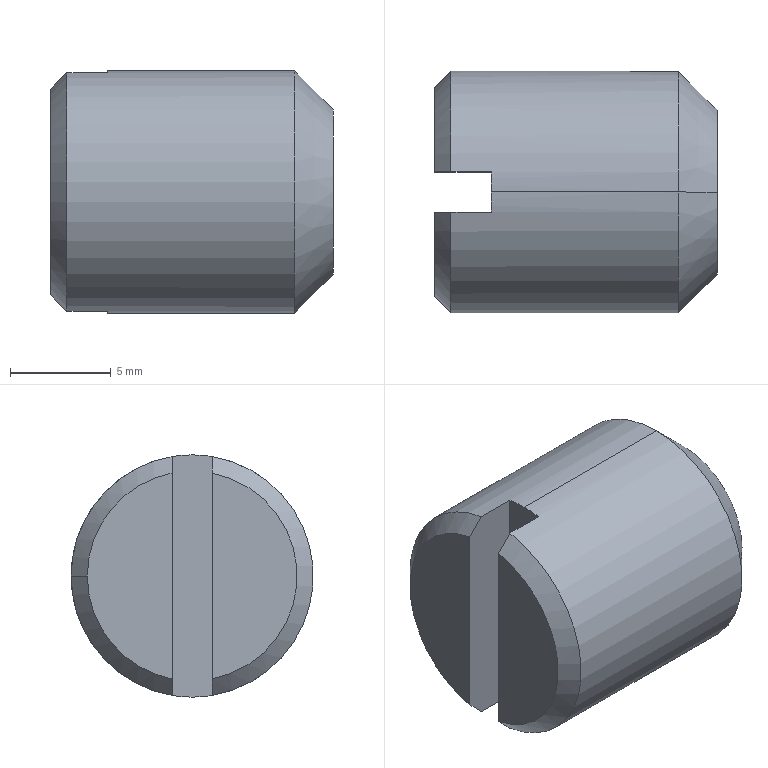Part | STEP file | 1 solid | 13 faces | box 14 x 12 x 12 mm | volume 1443 mm3 | plane 6 | cone 5 | cylinder 2 | commonest cylinder face diameters 12 x2
STEP:
#1=CARTESIAN_POINT('',(0.,0.,0.));
#2=DIRECTION('',(0.,0.,1.));
#3=DIRECTION('',(1.,0.,0.));
#4=AXIS2_PLACEMENT_3D('',#1,#2,#3);
#5=CARTESIAN_POINT('',(0.,1.,-5.099));
#6=VERTEX_POINT('',#5);
#7=CARTESIAN_POINT('',(0.,1.,5.099));
#8=VERTEX_POINT('',#7);
#9=CARTESIAN_POINT('',(0.,1.,-50.));
#10=DIRECTION('',(0.,0.,1.));
#11=VECTOR('',#10,1.);
#12=LINE('',#9,#11);
#13=CARTESIAN_POINT('',(0.,5.196,0.));
#14=DIRECTION('',(1.,0.,0.));
#15=DIRECTION('',(0.,1.,0.));
#16=AXIS2_PLACEMENT_3D('',#13,#14,#15);
#17=PLANE('',#16);
#18=CARTESIAN_POINT('',(-4.196,-50.));
#19=DIRECTION('',(0.,1.));
#20=VECTOR('',#19,1.);
#21=LINE('',#18,#20);
#22=(GEOMETRIC_REPRESENTATION_CONTEXT(2)PARAMETRIC_REPRESENTATION_CONTEXT()REPRESENTATION_CONTEXT('',''));
#23=DEFINITIONAL_REPRESENTATION('',(#21),#22);
#24=PCURVE('',#17,#23);
#25=CARTESIAN_POINT('',(0.,1.,-50.));
#26=DIRECTION('',(0.,1.,0.));
#27=DIRECTION('',(1.,0.,0.));
#28=AXIS2_PLACEMENT_3D('',#25,#26,#27);
#29=PLANE('',#28);
#30=CARTESIAN_POINT('',(0.,0.));
#31=DIRECTION('',(0.,-1.));
#32=VECTOR('',#31,1.);
#33=LINE('',#30,#32);
#34=(GEOMETRIC_REPRESENTATION_CONTEXT(2)PARAMETRIC_REPRESENTATION_CONTEXT()REPRESENTATION_CONTEXT('',''));
#35=DEFINITIONAL_REPRESENTATION('',(#33),#34);
#36=PCURVE('',#29,#35);
#37=SURFACE_CURVE('',#12,(#24,#36),.PCURVE_S1.);
#38=EDGE_CURVE('',#6,#8,#37,.T.);
#39=ORIENTED_EDGE('',*,*,#38,.T.);
#40=CARTESIAN_POINT('',(0.,5.196,0.));
#41=VERTEX_POINT('',#40);
#42=CARTESIAN_POINT('',(0.,0.,0.));
#43=DIRECTION('',(1.,0.,0.));
#44=DIRECTION('',(0.,1.,0.));
#45=AXIS2_PLACEMENT_3D('',#42,#43,#44);
#46=CIRCLE('',#45,5.196);
#47=CARTESIAN_POINT('',(-5.196,0.));
#48=DIRECTION('',(1.,0.));
#49=AXIS2_PLACEMENT_2D('',#47,#48);
#50=CIRCLE('',#49,5.196);
#51=(GEOMETRIC_REPRESENTATION_CONTEXT(2)PARAMETRIC_REPRESENTATION_CONTEXT()REPRESENTATION_CONTEXT('',''));
#52=DEFINITIONAL_REPRESENTATION('',(#50),#51);
#53=PCURVE('',#17,#52);
#54=CARTESIAN_POINT('',(0.804,0.,0.));
#55=DIRECTION('',(1.,0.,0.));
#56=DIRECTION('',(0.,1.,0.));
#57=AXIS2_PLACEMENT_3D('',#54,#55,#56);
#58=CONICAL_SURFACE('',#57,6.,0.7854);
#59=CARTESIAN_POINT('',(0.,-0.804));
#60=DIRECTION('',(1.,0.));
#61=VECTOR('',#60,1.);
#62=LINE('',#59,#61);
#63=(GEOMETRIC_REPRESENTATION_CONTEXT(2)PARAMETRIC_REPRESENTATION_CONTEXT()REPRESENTATION_CONTEXT('',''));
#64=DEFINITIONAL_REPRESENTATION('',(#62),#63);
#65=PCURVE('',#58,#64);
#66=SURFACE_CURVE('',#46,(#53,#65),.PCURVE_S1.);
#67=EDGE_CURVE('',#41,#8,#66,.T.);
#68=ORIENTED_EDGE('',*,*,#67,.F.);
#69=CARTESIAN_POINT('',(0.,0.,0.));
#70=DIRECTION('',(1.,0.,0.));
#71=DIRECTION('',(0.,1.,0.));
#72=AXIS2_PLACEMENT_3D('',#69,#70,#71);
#73=CIRCLE('',#72,5.196);
#74=CARTESIAN_POINT('',(-5.196,0.));
#75=DIRECTION('',(1.,0.));
#76=AXIS2_PLACEMENT_2D('',#74,#75);
#77=CIRCLE('',#76,5.196);
#78=(GEOMETRIC_REPRESENTATION_CONTEXT(2)PARAMETRIC_REPRESENTATION_CONTEXT()REPRESENTATION_CONTEXT('',''));
#79=DEFINITIONAL_REPRESENTATION('',(#77),#78);
#80=PCURVE('',#17,#79);
#81=CARTESIAN_POINT('',(0.804,0.,0.));
#82=DIRECTION('',(1.,0.,0.));
#83=DIRECTION('',(0.,1.,0.));
#84=AXIS2_PLACEMENT_3D('',#81,#82,#83);
#85=CONICAL_SURFACE('',#84,6.,0.7854);
#86=CARTESIAN_POINT('',(0.,-0.804));
#87=DIRECTION('',(1.,0.));
#88=VECTOR('',#87,1.);
#89=LINE('',#86,#88);
#90=(GEOMETRIC_REPRESENTATION_CONTEXT(2)PARAMETRIC_REPRESENTATION_CONTEXT()REPRESENTATION_CONTEXT('',''));
#91=DEFINITIONAL_REPRESENTATION('',(#89),#90);
#92=PCURVE('',#85,#91);
#93=SURFACE_CURVE('',#73,(#80,#92),.PCURVE_S1.);
#94=EDGE_CURVE('',#6,#41,#93,.T.);
#95=ORIENTED_EDGE('',*,*,#94,.F.);
#96=EDGE_LOOP('',(#39,#68,#95));
#97=FACE_BOUND('',#96,.T.);
#98=ADVANCED_FACE('',(#97),#17,.F.);
#99=CARTESIAN_POINT('',(14.,0.,4.07));
#100=VERTEX_POINT('',#99);
#101=CARTESIAN_POINT('',(14.,0.,-4.07));
#102=VERTEX_POINT('',#101);
#103=CARTESIAN_POINT('',(14.,0.,0.));
#104=DIRECTION('',(-1.,0.,0.));
#105=DIRECTION('',(0.,0.,1.));
#106=AXIS2_PLACEMENT_3D('',#103,#104,#105);
#107=CIRCLE('',#106,4.07);
#108=CARTESIAN_POINT('',(14.,0.,0.));
#109=DIRECTION('',(-1.,0.,0.));
#110=DIRECTION('',(0.,0.,1.));
#111=AXIS2_PLACEMENT_3D('',#108,#109,#110);
#112=PLANE('',#111);
#113=CARTESIAN_POINT('',(0.,0.));
#114=DIRECTION('',(1.,0.));
#115=AXIS2_PLACEMENT_2D('',#113,#114);
#116=CIRCLE('',#115,4.07);
#117=(GEOMETRIC_REPRESENTATION_CONTEXT(2)PARAMETRIC_REPRESENTATION_CONTEXT()REPRESENTATION_CONTEXT('',''));
#118=DEFINITIONAL_REPRESENTATION('',(#116),#117);
#119=PCURVE('',#112,#118);
#120=CARTESIAN_POINT('',(12.07,0.,0.));
#121=DIRECTION('',(-1.,0.,0.));
#122=DIRECTION('',(0.,0.,1.));
#123=AXIS2_PLACEMENT_3D('',#120,#121,#122);
#124=CONICAL_SURFACE('',#123,6.,0.7854);
#125=CARTESIAN_POINT('',(0.,-1.93));
#126=DIRECTION('',(1.,0.));
#127=VECTOR('',#126,1.);
#128=LINE('',#125,#127);
#129=(GEOMETRIC_REPRESENTATION_CONTEXT(2)PARAMETRIC_REPRESENTATION_CONTEXT()REPRESENTATION_CONTEXT('',''));
#130=DEFINITIONAL_REPRESENTATION('',(#128),#129);
#131=PCURVE('',#124,#130);
#132=SURFACE_CURVE('',#107,(#119,#131),.PCURVE_S1.);
#133=EDGE_CURVE('',#100,#102,#132,.T.);
#134=ORIENTED_EDGE('',*,*,#133,.F.);
#135=CARTESIAN_POINT('',(14.,0.,0.));
#136=DIRECTION('',(-1.,0.,0.));
#137=DIRECTION('',(0.,0.,1.));
#138=AXIS2_PLACEMENT_3D('',#135,#136,#137);
#139=CIRCLE('',#138,4.07);
#140=CARTESIAN_POINT('',(0.,0.));
#141=DIRECTION('',(1.,0.));
#142=AXIS2_PLACEMENT_2D('',#140,#141);
#143=CIRCLE('',#142,4.07);
#144=(GEOMETRIC_REPRESENTATION_CONTEXT(2)PARAMETRIC_REPRESENTATION_CONTEXT()REPRESENTATION_CONTEXT('',''));
#145=DEFINITIONAL_REPRESENTATION('',(#143),#144);
#146=PCURVE('',#112,#145);
#147=CARTESIAN_POINT('',(12.07,0.,0.));
#148=DIRECTION('',(-1.,0.,0.));
#149=DIRECTION('',(0.,0.,1.));
#150=AXIS2_PLACEMENT_3D('',#147,#148,#149);
#151=CONICAL_SURFACE('',#150,6.,0.7854);
#152=CARTESIAN_POINT('',(0.,-1.93));
#153=DIRECTION('',(1.,0.));
#154=VECTOR('',#153,1.);
#155=LINE('',#152,#154);
#156=(GEOMETRIC_REPRESENTATION_CONTEXT(2)PARAMETRIC_REPRESENTATION_CONTEXT()REPRESENTATION_CONTEXT('',''));
#157=DEFINITIONAL_REPRESENTATION('',(#155),#156);
#158=PCURVE('',#151,#157);
#159=SURFACE_CURVE('',#139,(#146,#158),.PCURVE_S1.);
#160=EDGE_CURVE('',#102,#100,#159,.T.);
#161=ORIENTED_EDGE('',*,*,#160,.F.);
#162=EDGE_LOOP('',(#134,#161));
#163=FACE_BOUND('',#162,.T.);
#164=ADVANCED_FACE('',(#163),#112,.F.);
#165=CARTESIAN_POINT('',(0.804,6.,0.));
#166=VERTEX_POINT('',#165);
#167=CARTESIAN_POINT('',(0.804,6.,0.));
#168=DIRECTION('',(0.7071,0.7071,0.));
#169=VECTOR('',#168,1.);
#170=LINE('',#167,#169);
#171=CARTESIAN_POINT('',(0.,0.));
#172=DIRECTION('',(0.,1.));
#173=VECTOR('',#172,1.);
#174=LINE('',#171,#173);
#175=(GEOMETRIC_REPRESENTATION_CONTEXT(2)PARAMETRIC_REPRESENTATION_CONTEXT()REPRESENTATION_CONTEXT('',''));
#176=DEFINITIONAL_REPRESENTATION('',(#174),#175);
#177=PCURVE('',#58,#176);
#178=CARTESIAN_POINT('',(6.283,0.));
#179=DIRECTION('',(0.,1.));
#180=VECTOR('',#179,1.);
#181=LINE('',#178,#180);
#182=(GEOMETRIC_REPRESENTATION_CONTEXT(2)PARAMETRIC_REPRESENTATION_CONTEXT()REPRESENTATION_CONTEXT('',''));
#183=DEFINITIONAL_REPRESENTATION('',(#181),#182);
#184=PCURVE('',#85,#183);
#185=SURFACE_CURVE('',#170,(#177,#184),.PCURVE_S1.);
#186=EDGE_CURVE('',#41,#166,#185,.T.);
#187=ORIENTED_EDGE('',*,*,#186,.F.);
#188=ORIENTED_EDGE('',*,*,#67,.T.);
#189=CARTESIAN_POINT('',(0.804,1.,5.916));
#190=VERTEX_POINT('',#189);
#191=CARTESIAN_POINT('',(0.,1.,5.099));
#192=CARTESIAN_POINT('',(0.2677,1.,5.372));
#193=CARTESIAN_POINT('',(0.5357,1.,5.644));
#194=CARTESIAN_POINT('',(0.804,1.,5.916));
#195=B_SPLINE_CURVE_WITH_KNOTS('',3,(#191,#192,#193,#194),.UNSPECIFIED.,.F.,.F.,(4,4),(0.,0.001146),.PIECEWISE_BEZIER_KNOTS.);
#196=CARTESIAN_POINT('',(1.377,-0.804));
#197=CARTESIAN_POINT('',(1.378,-0.7918));
#198=CARTESIAN_POINT('',(1.379,-0.7675));
#199=CARTESIAN_POINT('',(1.38,-0.731));
#200=CARTESIAN_POINT('',(1.381,-0.6945));
#201=CARTESIAN_POINT('',(1.382,-0.658));
#202=CARTESIAN_POINT('',(1.384,-0.6215));
#203=CARTESIAN_POINT('',(1.385,-0.5849));
#204=CARTESIAN_POINT('',(1.386,-0.5484));
#205=CARTESIAN_POINT('',(1.388,-0.5119));
#206=CARTESIAN_POINT('',(1.389,-0.4753));
#207=CARTESIAN_POINT('',(1.39,-0.4388));
#208=CARTESIAN_POINT('',(1.391,-0.4022));
#209=CARTESIAN_POINT('',(1.392,-0.3657));
#210=CARTESIAN_POINT('',(1.394,-0.3291));
#211=CARTESIAN_POINT('',(1.395,-0.2926));
#212=CARTESIAN_POINT('',(1.396,-0.256));
#213=CARTESIAN_POINT('',(1.397,-0.2195));
#214=CARTESIAN_POINT('',(1.398,-0.1829));
#215=CARTESIAN_POINT('',(1.399,-0.1463));
#216=CARTESIAN_POINT('',(1.4,-0.1097));
#217=CARTESIAN_POINT('',(1.401,-0.07317));
#218=CARTESIAN_POINT('',(1.402,-0.03659));
#219=CARTESIAN_POINT('',(1.403,-0.0122));
#220=CARTESIAN_POINT('',(1.403,0.));
#221=B_SPLINE_CURVE_WITH_KNOTS('',3,(#196,#197,#198,#199,#200,#201,#202,#203,#204,#205,#206,#207,#208,#209,#210,#211,#212,#213,#214,#215,#216,#217,#218,#219,#220),.UNSPECIFIED.,.F.,.F.,(4,1,1,1,1,1,1,1,1,1,1,1,1,1,1,1,1,1,1,1,1,1,4),(0.,0.00005211,0.0001042,0.0001563,0.0002084,0.0002605,0.0003127,0.0003648,0.0004169,0.000469,0.0005211,0.0005732,0.0006253,0.0006774,0.0007295,0.0007816,0.0008338,0.0008859,0.000938,0.0009901,0.001042,0.001094,0.001146),.QUASI_UNIFORM_KNOTS.);
#222=(GEOMETRIC_REPRESENTATION_CONTEXT(2)PARAMETRIC_REPRESENTATION_CONTEXT()REPRESENTATION_CONTEXT('',''));
#223=DEFINITIONAL_REPRESENTATION('',(#221),#222);
#224=PCURVE('',#58,#223);
#225=CARTESIAN_POINT('',(0.,-55.099));
#226=CARTESIAN_POINT('',(0.2677,-55.372));
#227=CARTESIAN_POINT('',(0.5357,-55.644));
#228=CARTESIAN_POINT('',(0.804,-55.916));
#229=B_SPLINE_CURVE_WITH_KNOTS('',3,(#225,#226,#227,#228),.UNSPECIFIED.,.F.,.F.,(4,4),(0.,0.001146),.PIECEWISE_BEZIER_KNOTS.);
#230=(GEOMETRIC_REPRESENTATION_CONTEXT(2)PARAMETRIC_REPRESENTATION_CONTEXT()REPRESENTATION_CONTEXT('',''));
#231=DEFINITIONAL_REPRESENTATION('',(#229),#230);
#232=PCURVE('',#29,#231);
#233=SURFACE_CURVE('',#195,(#224,#232),.PCURVE_S1.);
#234=EDGE_CURVE('',#8,#190,#233,.T.);
#235=ORIENTED_EDGE('',*,*,#234,.T.);
#236=CARTESIAN_POINT('',(0.804,0.,0.));
#237=DIRECTION('',(1.,0.,0.));
#238=DIRECTION('',(0.,0.,1.));
#239=AXIS2_PLACEMENT_3D('',#236,#237,#238);
#240=CIRCLE('',#239,6.);
#241=CARTESIAN_POINT('',(-4.712,0.));
#242=DIRECTION('',(1.,0.));
#243=VECTOR('',#242,1.);
#244=LINE('',#241,#243);
#245=(GEOMETRIC_REPRESENTATION_CONTEXT(2)PARAMETRIC_REPRESENTATION_CONTEXT()REPRESENTATION_CONTEXT('',''));
#246=DEFINITIONAL_REPRESENTATION('',(#244),#245);
#247=PCURVE('',#58,#246);
#248=CARTESIAN_POINT('',(-0.5499,0.,0.));
#249=DIRECTION('',(-1.,0.,0.));
#250=DIRECTION('',(0.,0.,1.));
#251=AXIS2_PLACEMENT_3D('',#248,#249,#250);
#252=CYLINDRICAL_SURFACE('',#251,6.);
#253=CARTESIAN_POINT('',(6.283,-1.354));
#254=DIRECTION('',(-1.,0.));
#255=VECTOR('',#254,1.);
#256=LINE('',#253,#255);
#257=(GEOMETRIC_REPRESENTATION_CONTEXT(2)PARAMETRIC_REPRESENTATION_CONTEXT()REPRESENTATION_CONTEXT('',''));
#258=DEFINITIONAL_REPRESENTATION('',(#256),#257);
#259=PCURVE('',#252,#258);
#260=SURFACE_CURVE('',#240,(#247,#259),.PCURVE_S1.);
#261=EDGE_CURVE('',#166,#190,#260,.T.);
#262=ORIENTED_EDGE('',*,*,#261,.F.);
#263=EDGE_LOOP('',(#187,#188,#235,#262));
#264=FACE_BOUND('',#263,.T.);
#265=ADVANCED_FACE('',(#264),#58,.T.);
#266=CARTESIAN_POINT('',(2.8,1.,5.916));
#267=VERTEX_POINT('',#266);
#268=CARTESIAN_POINT('',(-0.5499,1.,5.916));
#269=DIRECTION('',(1.,0.,0.));
#270=VECTOR('',#269,1.);
#271=LINE('',#268,#270);
#272=CARTESIAN_POINT('',(-0.5499,-55.916));
#273=DIRECTION('',(1.,0.));
#274=VECTOR('',#273,1.);
#275=LINE('',#272,#274);
#276=(GEOMETRIC_REPRESENTATION_CONTEXT(2)PARAMETRIC_REPRESENTATION_CONTEXT()REPRESENTATION_CONTEXT('',''));
#277=DEFINITIONAL_REPRESENTATION('',(#275),#276);
#278=PCURVE('',#29,#277);
#279=CARTESIAN_POINT('',(0.1674,0.));
#280=DIRECTION('',(0.,-1.));
#281=VECTOR('',#280,1.);
#282=LINE('',#279,#281);
#283=(GEOMETRIC_REPRESENTATION_CONTEXT(2)PARAMETRIC_REPRESENTATION_CONTEXT()REPRESENTATION_CONTEXT('',''));
#284=DEFINITIONAL_REPRESENTATION('',(#282),#283);
#285=PCURVE('',#252,#284);
#286=SURFACE_CURVE('',#271,(#278,#285),.PCURVE_S1.);
#287=EDGE_CURVE('',#190,#267,#286,.T.);
#288=ORIENTED_EDGE('',*,*,#287,.F.);
#289=ORIENTED_EDGE('',*,*,#234,.F.);
#290=ORIENTED_EDGE('',*,*,#38,.F.);
#291=CARTESIAN_POINT('',(0.804,1.,-5.916));
#292=VERTEX_POINT('',#291);
#293=CARTESIAN_POINT('',(0.804,1.,-5.916));
#294=CARTESIAN_POINT('',(0.5357,1.,-5.644));
#295=CARTESIAN_POINT('',(0.2677,1.,-5.372));
#296=CARTESIAN_POINT('',(0.,1.,-5.099));
#297=B_SPLINE_CURVE_WITH_KNOTS('',3,(#293,#294,#295,#296),.UNSPECIFIED.,.F.,.F.,(4,4),(0.,0.001146),.PIECEWISE_BEZIER_KNOTS.);
#298=CARTESIAN_POINT('',(0.804,-44.084));
#299=CARTESIAN_POINT('',(0.5357,-44.356));
#300=CARTESIAN_POINT('',(0.2677,-44.628));
#301=CARTESIAN_POINT('',(0.,-44.901));
#302=B_SPLINE_CURVE_WITH_KNOTS('',3,(#298,#299,#300,#301),.UNSPECIFIED.,.F.,.F.,(4,4),(0.,0.001146),.PIECEWISE_BEZIER_KNOTS.);
#303=(GEOMETRIC_REPRESENTATION_CONTEXT(2)PARAMETRIC_REPRESENTATION_CONTEXT()REPRESENTATION_CONTEXT('',''));
#304=DEFINITIONAL_REPRESENTATION('',(#302),#303);
#305=PCURVE('',#29,#304);
#306=CARTESIAN_POINT('',(4.88,0.));
#307=CARTESIAN_POINT('',(4.88,-0.0122));
#308=CARTESIAN_POINT('',(4.881,-0.03659));
#309=CARTESIAN_POINT('',(4.882,-0.07317));
#310=CARTESIAN_POINT('',(4.883,-0.1097));
#311=CARTESIAN_POINT('',(4.884,-0.1463));
#312=CARTESIAN_POINT('',(4.885,-0.1829));
#313=CARTESIAN_POINT('',(4.886,-0.2195));
#314=CARTESIAN_POINT('',(4.887,-0.256));
#315=CARTESIAN_POINT('',(4.889,-0.2926));
#316=CARTESIAN_POINT('',(4.89,-0.3291));
#317=CARTESIAN_POINT('',(4.891,-0.3657));
#318=CARTESIAN_POINT('',(4.892,-0.4022));
#319=CARTESIAN_POINT('',(4.893,-0.4388));
#320=CARTESIAN_POINT('',(4.894,-0.4753));
#321=CARTESIAN_POINT('',(4.896,-0.5119));
#322=CARTESIAN_POINT('',(4.897,-0.5484));
#323=CARTESIAN_POINT('',(4.898,-0.5849));
#324=CARTESIAN_POINT('',(4.899,-0.6215));
#325=CARTESIAN_POINT('',(4.901,-0.658));
#326=CARTESIAN_POINT('',(4.902,-0.6945));
#327=CARTESIAN_POINT('',(4.903,-0.731));
#328=CARTESIAN_POINT('',(4.905,-0.7675));
#329=CARTESIAN_POINT('',(4.906,-0.7918));
#330=CARTESIAN_POINT('',(4.906,-0.804));
#331=B_SPLINE_CURVE_WITH_KNOTS('',3,(#306,#307,#308,#309,#310,#311,#312,#313,#314,#315,#316,#317,#318,#319,#320,#321,#322,#323,#324,#325,#326,#327,#328,#329,#330),.UNSPECIFIED.,.F.,.F.,(4,1,1,1,1,1,1,1,1,1,1,1,1,1,1,1,1,1,1,1,1,1,4),(0.,0.00005211,0.0001042,0.0001563,0.0002084,0.0002605,0.0003127,0.0003648,0.0004169,0.000469,0.0005211,0.0005732,0.0006253,0.0006774,0.0007295,0.0007816,0.0008338,0.0008859,0.000938,0.0009901,0.001042,0.001094,0.001146),.QUASI_UNIFORM_KNOTS.);
#332=(GEOMETRIC_REPRESENTATION_CONTEXT(2)PARAMETRIC_REPRESENTATION_CONTEXT()REPRESENTATION_CONTEXT('',''));
#333=DEFINITIONAL_REPRESENTATION('',(#331),#332);
#334=PCURVE('',#85,#333);
#335=SURFACE_CURVE('',#297,(#305,#334),.PCURVE_S1.);
#336=EDGE_CURVE('',#292,#6,#335,.T.);
#337=ORIENTED_EDGE('',*,*,#336,.F.);
#338=CARTESIAN_POINT('',(2.8,1.,-5.916));
#339=VERTEX_POINT('',#338);
#340=CARTESIAN_POINT('',(-0.5499,1.,-5.916));
#341=DIRECTION('',(-1.,0.,0.));
#342=VECTOR('',#341,1.);
#343=LINE('',#340,#342);
#344=CARTESIAN_POINT('',(-0.5499,-44.084));
#345=DIRECTION('',(-1.,0.));
#346=VECTOR('',#345,1.);
#347=LINE('',#344,#346);
#348=(GEOMETRIC_REPRESENTATION_CONTEXT(2)PARAMETRIC_REPRESENTATION_CONTEXT()REPRESENTATION_CONTEXT('',''));
#349=DEFINITIONAL_REPRESENTATION('',(#347),#348);
#350=PCURVE('',#29,#349);
#351=CARTESIAN_POINT('',(2.974,0.));
#352=DIRECTION('',(0.,1.));
#353=VECTOR('',#352,1.);
#354=LINE('',#351,#353);
#355=(GEOMETRIC_REPRESENTATION_CONTEXT(2)PARAMETRIC_REPRESENTATION_CONTEXT()REPRESENTATION_CONTEXT('',''));
#356=DEFINITIONAL_REPRESENTATION('',(#354),#355);
#357=PCURVE('',#252,#356);
#358=SURFACE_CURVE('',#343,(#350,#357),.PCURVE_S1.);
#359=EDGE_CURVE('',#339,#292,#358,.T.);
#360=ORIENTED_EDGE('',*,*,#359,.F.);
#361=CARTESIAN_POINT('',(2.8,1.,-50.));
#362=DIRECTION('',(0.,0.,1.));
#363=VECTOR('',#362,1.);
#364=LINE('',#361,#363);
#365=CARTESIAN_POINT('',(2.8,0.));
#366=DIRECTION('',(0.,-1.));
#367=VECTOR('',#366,1.);
#368=LINE('',#365,#367);
#369=(GEOMETRIC_REPRESENTATION_CONTEXT(2)PARAMETRIC_REPRESENTATION_CONTEXT()REPRESENTATION_CONTEXT('',''));
#370=DEFINITIONAL_REPRESENTATION('',(#368),#369);
#371=PCURVE('',#29,#370);
#372=CARTESIAN_POINT('',(2.8,-1.,-50.));
#373=DIRECTION('',(1.,0.,0.));
#374=DIRECTION('',(0.,1.,0.));
#375=AXIS2_PLACEMENT_3D('',#372,#373,#374);
#376=PLANE('',#375);
#377=CARTESIAN_POINT('',(2.,0.));
#378=DIRECTION('',(0.,1.));
#379=VECTOR('',#378,1.);
#380=LINE('',#377,#379);
#381=(GEOMETRIC_REPRESENTATION_CONTEXT(2)PARAMETRIC_REPRESENTATION_CONTEXT()REPRESENTATION_CONTEXT('',''));
#382=DEFINITIONAL_REPRESENTATION('',(#380),#381);
#383=PCURVE('',#376,#382);
#384=SURFACE_CURVE('',#364,(#371,#383),.PCURVE_S1.);
#385=EDGE_CURVE('',#339,#267,#384,.T.);
#386=ORIENTED_EDGE('',*,*,#385,.T.);
#387=EDGE_LOOP('',(#288,#289,#290,#337,#360,#386));
#388=FACE_BOUND('',#387,.T.);
#389=ADVANCED_FACE('',(#388),#29,.F.);
#390=CARTESIAN_POINT('',(0.,-1.,5.099));
#391=VERTEX_POINT('',#390);
#392=CARTESIAN_POINT('',(0.,-1.,-5.099));
#393=VERTEX_POINT('',#392);
#394=CARTESIAN_POINT('',(0.,-1.,-50.));
#395=DIRECTION('',(0.,0.,-1.));
#396=VECTOR('',#395,1.);
#397=LINE('',#394,#396);
#398=CARTESIAN_POINT('',(0.,5.196,0.));
#399=DIRECTION('',(1.,0.,0.));
#400=DIRECTION('',(0.,1.,0.));
#401=AXIS2_PLACEMENT_3D('',#398,#399,#400);
#402=PLANE('',#401);
#403=CARTESIAN_POINT('',(-6.196,-50.));
#404=DIRECTION('',(0.,-1.));
#405=VECTOR('',#404,1.);
#406=LINE('',#403,#405);
#407=(GEOMETRIC_REPRESENTATION_CONTEXT(2)PARAMETRIC_REPRESENTATION_CONTEXT()REPRESENTATION_CONTEXT('',''));
#408=DEFINITIONAL_REPRESENTATION('',(#406),#407);
#409=PCURVE('',#402,#408);
#410=CARTESIAN_POINT('',(0.,-1.,-50.));
#411=DIRECTION('',(0.,-1.,0.));
#412=DIRECTION('',(0.,0.,-1.));
#413=AXIS2_PLACEMENT_3D('',#410,#411,#412);
#414=PLANE('',#413);
#415=CARTESIAN_POINT('',(0.,0.));
#416=DIRECTION('',(1.,0.));
#417=VECTOR('',#416,1.);
#418=LINE('',#415,#417);
#419=(GEOMETRIC_REPRESENTATION_CONTEXT(2)PARAMETRIC_REPRESENTATION_CONTEXT()REPRESENTATION_CONTEXT('',''));
#420=DEFINITIONAL_REPRESENTATION('',(#418),#419);
#421=PCURVE('',#414,#420);
#422=SURFACE_CURVE('',#397,(#409,#421),.PCURVE_S1.);
#423=EDGE_CURVE('',#391,#393,#422,.T.);
#424=ORIENTED_EDGE('',*,*,#423,.T.);
#425=CARTESIAN_POINT('',(0.,0.,0.));
#426=DIRECTION('',(1.,0.,0.));
#427=DIRECTION('',(0.,1.,0.));
#428=AXIS2_PLACEMENT_3D('',#425,#426,#427);
#429=CIRCLE('',#428,5.196);
#430=CARTESIAN_POINT('',(-5.196,0.));
#431=DIRECTION('',(1.,0.));
#432=AXIS2_PLACEMENT_2D('',#430,#431);
#433=CIRCLE('',#432,5.196);
#434=(GEOMETRIC_REPRESENTATION_CONTEXT(2)PARAMETRIC_REPRESENTATION_CONTEXT()REPRESENTATION_CONTEXT('',''));
#435=DEFINITIONAL_REPRESENTATION('',(#433),#434);
#436=PCURVE('',#402,#435);
#437=CARTESIAN_POINT('',(0.804,0.,0.));
#438=DIRECTION('',(1.,0.,0.));
#439=DIRECTION('',(0.,1.,0.));
#440=AXIS2_PLACEMENT_3D('',#437,#438,#439);
#441=CONICAL_SURFACE('',#440,6.,0.7854);
#442=CARTESIAN_POINT('',(0.,-0.804));
#443=DIRECTION('',(1.,0.));
#444=VECTOR('',#443,1.);
#445=LINE('',#442,#444);
#446=(GEOMETRIC_REPRESENTATION_CONTEXT(2)PARAMETRIC_REPRESENTATION_CONTEXT()REPRESENTATION_CONTEXT('',''));
#447=DEFINITIONAL_REPRESENTATION('',(#445),#446);
#448=PCURVE('',#441,#447);
#449=SURFACE_CURVE('',#429,(#436,#448),.PCURVE_S1.);
#450=EDGE_CURVE('',#391,#393,#449,.T.);
#451=ORIENTED_EDGE('',*,*,#450,.F.);
#452=EDGE_LOOP('',(#424,#451));
#453=FACE_BOUND('',#452,.T.);
#454=ADVANCED_FACE('',(#453),#402,.F.);
#455=CARTESIAN_POINT('',(2.8,-1.,-5.916));
#456=VERTEX_POINT('',#455);
#457=CARTESIAN_POINT('',(2.8,0.,-6.));
#458=VERTEX_POINT('',#457);
#459=CARTESIAN_POINT('',(2.8,0.,0.));
#460=DIRECTION('',(1.,0.,0.));
#461=DIRECTION('',(0.,0.,1.));
#462=AXIS2_PLACEMENT_3D('',#459,#460,#461);
#463=CIRCLE('',#462,6.);
#464=CARTESIAN_POINT('',(1.,50.));
#465=DIRECTION('',(0.,1.));
#466=AXIS2_PLACEMENT_2D('',#464,#465);
#467=CIRCLE('',#466,6.);
#468=(GEOMETRIC_REPRESENTATION_CONTEXT(2)PARAMETRIC_REPRESENTATION_CONTEXT()REPRESENTATION_CONTEXT('',''));
#469=DEFINITIONAL_REPRESENTATION('',(#467),#468);
#470=PCURVE('',#376,#469);
#471=CARTESIAN_POINT('',(-0.5499,0.,0.));
#472=DIRECTION('',(-1.,0.,0.));
#473=DIRECTION('',(0.,0.,1.));
#474=AXIS2_PLACEMENT_3D('',#471,#472,#473);
#475=CYLINDRICAL_SURFACE('',#474,6.);
#476=CARTESIAN_POINT('',(6.283,-3.35));
#477=DIRECTION('',(-1.,0.));
#478=VECTOR('',#477,1.);
#479=LINE('',#476,#478);
#480=(GEOMETRIC_REPRESENTATION_CONTEXT(2)PARAMETRIC_REPRESENTATION_CONTEXT()REPRESENTATION_CONTEXT('',''));
#481=DEFINITIONAL_REPRESENTATION('',(#479),#480);
#482=PCURVE('',#475,#481);
#483=SURFACE_CURVE('',#463,(#470,#482),.PCURVE_S1.);
#484=EDGE_CURVE('',#456,#458,#483,.T.);
#485=ORIENTED_EDGE('',*,*,#484,.F.);
#486=CARTESIAN_POINT('',(2.8,-1.,5.916));
#487=VERTEX_POINT('',#486);
#488=CARTESIAN_POINT('',(2.8,-1.,-50.));
#489=DIRECTION('',(0.,0.,1.));
#490=VECTOR('',#489,1.);
#491=LINE('',#488,#490);
#492=CARTESIAN_POINT('',(0.,0.));
#493=DIRECTION('',(0.,1.));
#494=VECTOR('',#493,1.);
#495=LINE('',#492,#494);
#496=(GEOMETRIC_REPRESENTATION_CONTEXT(2)PARAMETRIC_REPRESENTATION_CONTEXT()REPRESENTATION_CONTEXT('',''));
#497=DEFINITIONAL_REPRESENTATION('',(#495),#496);
#498=PCURVE('',#376,#497);
#499=CARTESIAN_POINT('',(0.,2.8));
#500=DIRECTION('',(-1.,0.));
#501=VECTOR('',#500,1.);
#502=LINE('',#499,#501);
#503=(GEOMETRIC_REPRESENTATION_CONTEXT(2)PARAMETRIC_REPRESENTATION_CONTEXT()REPRESENTATION_CONTEXT('',''));
#504=DEFINITIONAL_REPRESENTATION('',(#502),#503);
#505=PCURVE('',#414,#504);
#506=SURFACE_CURVE('',#491,(#498,#505),.PCURVE_S1.);
#507=EDGE_CURVE('',#456,#487,#506,.T.);
#508=ORIENTED_EDGE('',*,*,#507,.T.);
#509=CARTESIAN_POINT('',(2.8,0.,6.));
#510=VERTEX_POINT('',#509);
#511=CARTESIAN_POINT('',(2.8,0.,0.));
#512=DIRECTION('',(1.,0.,0.));
#513=DIRECTION('',(0.,0.,1.));
#514=AXIS2_PLACEMENT_3D('',#511,#512,#513);
#515=CIRCLE('',#514,6.);
#516=CARTESIAN_POINT('',(1.,50.));
#517=DIRECTION('',(0.,1.));
#518=AXIS2_PLACEMENT_2D('',#516,#517);
#519=CIRCLE('',#518,6.);
#520=(GEOMETRIC_REPRESENTATION_CONTEXT(2)PARAMETRIC_REPRESENTATION_CONTEXT()REPRESENTATION_CONTEXT('',''));
#521=DEFINITIONAL_REPRESENTATION('',(#519),#520);
#522=PCURVE('',#376,#521);
#523=CARTESIAN_POINT('',(6.283,-3.35));
#524=DIRECTION('',(-1.,0.));
#525=VECTOR('',#524,1.);
#526=LINE('',#523,#525);
#527=(GEOMETRIC_REPRESENTATION_CONTEXT(2)PARAMETRIC_REPRESENTATION_CONTEXT()REPRESENTATION_CONTEXT('',''));
#528=DEFINITIONAL_REPRESENTATION('',(#526),#527);
#529=PCURVE('',#475,#528);
#530=SURFACE_CURVE('',#515,(#522,#529),.PCURVE_S1.);
#531=EDGE_CURVE('',#510,#487,#530,.T.);
#532=ORIENTED_EDGE('',*,*,#531,.F.);
#533=CARTESIAN_POINT('',(2.8,0.,0.));
#534=DIRECTION('',(1.,0.,0.));
#535=DIRECTION('',(0.,0.,1.));
#536=AXIS2_PLACEMENT_3D('',#533,#534,#535);
#537=CIRCLE('',#536,6.);
#538=CARTESIAN_POINT('',(1.,50.));
#539=DIRECTION('',(0.,1.));
#540=AXIS2_PLACEMENT_2D('',#538,#539);
#541=CIRCLE('',#540,6.);
#542=(GEOMETRIC_REPRESENTATION_CONTEXT(2)PARAMETRIC_REPRESENTATION_CONTEXT()REPRESENTATION_CONTEXT('',''));
#543=DEFINITIONAL_REPRESENTATION('',(#541),#542);
#544=PCURVE('',#376,#543);
#545=CARTESIAN_POINT('',(6.283,-3.35));
#546=DIRECTION('',(-1.,0.));
#547=VECTOR('',#546,1.);
#548=LINE('',#545,#547);
#549=(GEOMETRIC_REPRESENTATION_CONTEXT(2)PARAMETRIC_REPRESENTATION_CONTEXT()REPRESENTATION_CONTEXT('',''));
#550=DEFINITIONAL_REPRESENTATION('',(#548),#549);
#551=PCURVE('',#252,#550);
#552=SURFACE_CURVE('',#537,(#544,#551),.PCURVE_S1.);
#553=EDGE_CURVE('',#267,#510,#552,.T.);
#554=ORIENTED_EDGE('',*,*,#553,.F.);
#555=ORIENTED_EDGE('',*,*,#385,.F.);
#556=CARTESIAN_POINT('',(2.8,0.,0.));
#557=DIRECTION('',(1.,0.,0.));
#558=DIRECTION('',(0.,0.,1.));
#559=AXIS2_PLACEMENT_3D('',#556,#557,#558);
#560=CIRCLE('',#559,6.);
#561=CARTESIAN_POINT('',(1.,50.));
#562=DIRECTION('',(0.,1.));
#563=AXIS2_PLACEMENT_2D('',#561,#562);
#564=CIRCLE('',#563,6.);
#565=(GEOMETRIC_REPRESENTATION_CONTEXT(2)PARAMETRIC_REPRESENTATION_CONTEXT()REPRESENTATION_CONTEXT('',''));
#566=DEFINITIONAL_REPRESENTATION('',(#564),#565);
#567=PCURVE('',#376,#566);
#568=CARTESIAN_POINT('',(6.283,-3.35));
#569=DIRECTION('',(-1.,0.));
#570=VECTOR('',#569,1.);
#571=LINE('',#568,#570);
#572=(GEOMETRIC_REPRESENTATION_CONTEXT(2)PARAMETRIC_REPRESENTATION_CONTEXT()REPRESENTATION_CONTEXT('',''));
#573=DEFINITIONAL_REPRESENTATION('',(#571),#572);
#574=PCURVE('',#252,#573);
#575=SURFACE_CURVE('',#560,(#567,#574),.PCURVE_S1.);
#576=EDGE_CURVE('',#458,#339,#575,.T.);
#577=ORIENTED_EDGE('',*,*,#576,.F.);
#578=EDGE_LOOP('',(#485,#508,#532,#554,#555,#577));
#579=FACE_BOUND('',#578,.T.);
#580=ADVANCED_FACE('',(#579),#376,.F.);
#581=CARTESIAN_POINT('',(12.07,0.,-6.));
#582=VERTEX_POINT('',#581);
#583=CARTESIAN_POINT('',(12.07,0.,-6.));
#584=DIRECTION('',(-0.7071,0.,-0.7071));
#585=VECTOR('',#584,1.);
#586=LINE('',#583,#585);
#587=CARTESIAN_POINT('',(3.142,0.));
#588=DIRECTION('',(0.,1.));
#589=VECTOR('',#588,1.);
#590=LINE('',#587,#589);
#591=(GEOMETRIC_REPRESENTATION_CONTEXT(2)PARAMETRIC_REPRESENTATION_CONTEXT()REPRESENTATION_CONTEXT('',''));
#592=DEFINITIONAL_REPRESENTATION('',(#590),#591);
#593=PCURVE('',#151,#592);
#594=CARTESIAN_POINT('',(3.142,0.));
#595=DIRECTION('',(0.,1.));
#596=VECTOR('',#595,1.);
#597=LINE('',#594,#596);
#598=(GEOMETRIC_REPRESENTATION_CONTEXT(2)PARAMETRIC_REPRESENTATION_CONTEXT()REPRESENTATION_CONTEXT('',''));
#599=DEFINITIONAL_REPRESENTATION('',(#597),#598);
#600=PCURVE('',#124,#599);
#601=SURFACE_CURVE('',#586,(#593,#600),.PCURVE_S1.);
#602=EDGE_CURVE('',#102,#582,#601,.T.);
#603=ORIENTED_EDGE('',*,*,#602,.F.);
#604=ORIENTED_EDGE('',*,*,#160,.T.);
#605=CARTESIAN_POINT('',(12.07,0.,6.));
#606=VERTEX_POINT('',#605);
#607=CARTESIAN_POINT('',(12.07,0.,6.));
#608=DIRECTION('',(-0.7071,0.,0.7071));
#609=VECTOR('',#608,1.);
#610=LINE('',#607,#609);
#611=CARTESIAN_POINT('',(6.283,0.));
#612=DIRECTION('',(0.,1.));
#613=VECTOR('',#612,1.);
#614=LINE('',#611,#613);
#615=(GEOMETRIC_REPRESENTATION_CONTEXT(2)PARAMETRIC_REPRESENTATION_CONTEXT()REPRESENTATION_CONTEXT('',''));
#616=DEFINITIONAL_REPRESENTATION('',(#614),#615);
#617=PCURVE('',#151,#616);
#618=CARTESIAN_POINT('',(0.,0.));
#619=DIRECTION('',(0.,1.));
#620=VECTOR('',#619,1.);
#621=LINE('',#618,#620);
#622=(GEOMETRIC_REPRESENTATION_CONTEXT(2)PARAMETRIC_REPRESENTATION_CONTEXT()REPRESENTATION_CONTEXT('',''));
#623=DEFINITIONAL_REPRESENTATION('',(#621),#622);
#624=PCURVE('',#124,#623);
#625=SURFACE_CURVE('',#610,(#617,#624),.PCURVE_S1.);
#626=EDGE_CURVE('',#100,#606,#625,.T.);
#627=ORIENTED_EDGE('',*,*,#626,.T.);
#628=CARTESIAN_POINT('',(12.07,0.,0.));
#629=DIRECTION('',(-1.,0.,0.));
#630=DIRECTION('',(0.,0.,1.));
#631=AXIS2_PLACEMENT_3D('',#628,#629,#630);
#632=CIRCLE('',#631,6.);
#633=CARTESIAN_POINT('',(0.,0.));
#634=DIRECTION('',(1.,0.));
#635=VECTOR('',#634,1.);
#636=LINE('',#633,#635);
#637=(GEOMETRIC_REPRESENTATION_CONTEXT(2)PARAMETRIC_REPRESENTATION_CONTEXT()REPRESENTATION_CONTEXT('',''));
#638=DEFINITIONAL_REPRESENTATION('',(#636),#637);
#639=PCURVE('',#151,#638);
#640=CARTESIAN_POINT('',(0.,-12.62));
#641=DIRECTION('',(1.,0.));
#642=VECTOR('',#641,1.);
#643=LINE('',#640,#642);
#644=(GEOMETRIC_REPRESENTATION_CONTEXT(2)PARAMETRIC_REPRESENTATION_CONTEXT()REPRESENTATION_CONTEXT('',''));
#645=DEFINITIONAL_REPRESENTATION('',(#643),#644);
#646=PCURVE('',#475,#645);
#647=SURFACE_CURVE('',#632,(#639,#646),.PCURVE_S1.);
#648=EDGE_CURVE('',#582,#606,#647,.T.);
#649=ORIENTED_EDGE('',*,*,#648,.F.);
#650=EDGE_LOOP('',(#603,#604,#627,#649));
#651=FACE_BOUND('',#650,.T.);
#652=ADVANCED_FACE('',(#651),#151,.T.);
#653=ORIENTED_EDGE('',*,*,#450,.T.);
#654=CARTESIAN_POINT('',(0.804,-1.,-5.916));
#655=VERTEX_POINT('',#654);
#656=CARTESIAN_POINT('',(0.,-1.,-5.099));
#657=CARTESIAN_POINT('',(0.2677,-1.,-5.372));
#658=CARTESIAN_POINT('',(0.5357,-1.,-5.644));
#659=CARTESIAN_POINT('',(0.804,-1.,-5.916));
#660=B_SPLINE_CURVE_WITH_KNOTS('',3,(#656,#657,#658,#659),.UNSPECIFIED.,.F.,.F.,(4,4),(0.,0.001146),.PIECEWISE_BEZIER_KNOTS.);
#661=CARTESIAN_POINT('',(4.519,-0.804));
#662=CARTESIAN_POINT('',(4.519,-0.7918));
#663=CARTESIAN_POINT('',(4.52,-0.7675));
#664=CARTESIAN_POINT('',(4.521,-0.731));
#665=CARTESIAN_POINT('',(4.523,-0.6945));
#666=CARTESIAN_POINT('',(4.524,-0.658));
#667=CARTESIAN_POINT('',(4.525,-0.6215));
#668=CARTESIAN_POINT('',(4.527,-0.5849));
#669=CARTESIAN_POINT('',(4.528,-0.5484));
#670=CARTESIAN_POINT('',(4.529,-0.5119));
#671=CARTESIAN_POINT('',(4.53,-0.4753));
#672=CARTESIAN_POINT('',(4.532,-0.4388));
#673=CARTESIAN_POINT('',(4.533,-0.4022));
#674=CARTESIAN_POINT('',(4.534,-0.3657));
#675=CARTESIAN_POINT('',(4.535,-0.3291));
#676=CARTESIAN_POINT('',(4.536,-0.2926));
#677=CARTESIAN_POINT('',(4.537,-0.256));
#678=CARTESIAN_POINT('',(4.539,-0.2195));
#679=CARTESIAN_POINT('',(4.54,-0.1829));
#680=CARTESIAN_POINT('',(4.541,-0.1463));
#681=CARTESIAN_POINT('',(4.542,-0.1097));
#682=CARTESIAN_POINT('',(4.543,-0.07317));
#683=CARTESIAN_POINT('',(4.544,-0.03659));
#684=CARTESIAN_POINT('',(4.545,-0.0122));
#685=CARTESIAN_POINT('',(4.545,0.));
#686=B_SPLINE_CURVE_WITH_KNOTS('',3,(#661,#662,#663,#664,#665,#666,#667,#668,#669,#670,#671,#672,#673,#674,#675,#676,#677,#678,#679,#680,#681,#682,#683,#684,#685),.UNSPECIFIED.,.F.,.F.,(4,1,1,1,1,1,1,1,1,1,1,1,1,1,1,1,1,1,1,1,1,1,4),(0.,0.00005211,0.0001042,0.0001563,0.0002084,0.0002605,0.0003127,0.0003648,0.0004169,0.000469,0.0005211,0.0005732,0.0006253,0.0006774,0.0007295,0.0007816,0.0008338,0.0008859,0.000938,0.0009901,0.001042,0.001094,0.001146),.QUASI_UNIFORM_KNOTS.);
#687=(GEOMETRIC_REPRESENTATION_CONTEXT(2)PARAMETRIC_REPRESENTATION_CONTEXT()REPRESENTATION_CONTEXT('',''));
#688=DEFINITIONAL_REPRESENTATION('',(#686),#687);
#689=PCURVE('',#441,#688);
#690=CARTESIAN_POINT('',(-44.901,0.));
#691=CARTESIAN_POINT('',(-44.628,0.2677));
#692=CARTESIAN_POINT('',(-44.356,0.5357));
#693=CARTESIAN_POINT('',(-44.084,0.804));
#694=B_SPLINE_CURVE_WITH_KNOTS('',3,(#690,#691,#692,#693),.UNSPECIFIED.,.F.,.F.,(4,4),(0.,0.001146),.PIECEWISE_BEZIER_KNOTS.);
#695=(GEOMETRIC_REPRESENTATION_CONTEXT(2)PARAMETRIC_REPRESENTATION_CONTEXT()REPRESENTATION_CONTEXT('',''));
#696=DEFINITIONAL_REPRESENTATION('',(#694),#695);
#697=PCURVE('',#414,#696);
#698=SURFACE_CURVE('',#660,(#689,#697),.PCURVE_S1.);
#699=EDGE_CURVE('',#393,#655,#698,.T.);
#700=ORIENTED_EDGE('',*,*,#699,.T.);
#701=CARTESIAN_POINT('',(0.804,-1.,5.916));
#702=VERTEX_POINT('',#701);
#703=CARTESIAN_POINT('',(0.804,0.,0.));
#704=DIRECTION('',(1.,0.,0.));
#705=DIRECTION('',(0.,0.,1.));
#706=AXIS2_PLACEMENT_3D('',#703,#704,#705);
#707=CIRCLE('',#706,6.);
#708=CARTESIAN_POINT('',(1.571,0.));
#709=DIRECTION('',(1.,0.));
#710=VECTOR('',#709,1.);
#711=LINE('',#708,#710);
#712=(GEOMETRIC_REPRESENTATION_CONTEXT(2)PARAMETRIC_REPRESENTATION_CONTEXT()REPRESENTATION_CONTEXT('',''));
#713=DEFINITIONAL_REPRESENTATION('',(#711),#712);
#714=PCURVE('',#441,#713);
#715=CARTESIAN_POINT('',(6.283,-1.354));
#716=DIRECTION('',(-1.,0.));
#717=VECTOR('',#716,1.);
#718=LINE('',#715,#717);
#719=(GEOMETRIC_REPRESENTATION_CONTEXT(2)PARAMETRIC_REPRESENTATION_CONTEXT()REPRESENTATION_CONTEXT('',''));
#720=DEFINITIONAL_REPRESENTATION('',(#718),#719);
#721=PCURVE('',#475,#720);
#722=SURFACE_CURVE('',#707,(#714,#721),.PCURVE_S1.);
#723=EDGE_CURVE('',#702,#655,#722,.T.);
#724=ORIENTED_EDGE('',*,*,#723,.F.);
#725=CARTESIAN_POINT('',(0.804,-1.,5.916));
#726=CARTESIAN_POINT('',(0.5357,-1.,5.644));
#727=CARTESIAN_POINT('',(0.2677,-1.,5.372));
#728=CARTESIAN_POINT('',(0.,-1.,5.099));
#729=B_SPLINE_CURVE_WITH_KNOTS('',3,(#725,#726,#727,#728),.UNSPECIFIED.,.F.,.F.,(4,4),(0.,0.001146),.PIECEWISE_BEZIER_KNOTS.);
#730=CARTESIAN_POINT('',(1.738,0.));
#731=CARTESIAN_POINT('',(1.739,-0.0122));
#732=CARTESIAN_POINT('',(1.739,-0.03659));
#733=CARTESIAN_POINT('',(1.74,-0.07317));
#734=CARTESIAN_POINT('',(1.741,-0.1097));
#735=CARTESIAN_POINT('',(1.742,-0.1463));
#736=CARTESIAN_POINT('',(1.744,-0.1829));
#737=CARTESIAN_POINT('',(1.745,-0.2195));
#738=CARTESIAN_POINT('',(1.746,-0.256));
#739=CARTESIAN_POINT('',(1.747,-0.2926));
#740=CARTESIAN_POINT('',(1.748,-0.3291));
#741=CARTESIAN_POINT('',(1.749,-0.3657));
#742=CARTESIAN_POINT('',(1.75,-0.4022));
#743=CARTESIAN_POINT('',(1.752,-0.4388));
#744=CARTESIAN_POINT('',(1.753,-0.4753));
#745=CARTESIAN_POINT('',(1.754,-0.5119));
#746=CARTESIAN_POINT('',(1.755,-0.5484));
#747=CARTESIAN_POINT('',(1.757,-0.5849));
#748=CARTESIAN_POINT('',(1.758,-0.6215));
#749=CARTESIAN_POINT('',(1.759,-0.658));
#750=CARTESIAN_POINT('',(1.76,-0.6945));
#751=CARTESIAN_POINT('',(1.762,-0.731));
#752=CARTESIAN_POINT('',(1.763,-0.7675));
#753=CARTESIAN_POINT('',(1.764,-0.7918));
#754=CARTESIAN_POINT('',(1.764,-0.804));
#755=B_SPLINE_CURVE_WITH_KNOTS('',3,(#730,#731,#732,#733,#734,#735,#736,#737,#738,#739,#740,#741,#742,#743,#744,#745,#746,#747,#748,#749,#750,#751,#752,#753,#754),.UNSPECIFIED.,.F.,.F.,(4,1,1,1,1,1,1,1,1,1,1,1,1,1,1,1,1,1,1,1,1,1,4),(0.,0.00005211,0.0001042,0.0001563,0.0002084,0.0002605,0.0003127,0.0003648,0.0004169,0.000469,0.0005211,0.0005732,0.0006253,0.0006774,0.0007295,0.0007816,0.0008338,0.0008859,0.000938,0.0009901,0.001042,0.001094,0.001146),.QUASI_UNIFORM_KNOTS.);
#756=(GEOMETRIC_REPRESENTATION_CONTEXT(2)PARAMETRIC_REPRESENTATION_CONTEXT()REPRESENTATION_CONTEXT('',''));
#757=DEFINITIONAL_REPRESENTATION('',(#755),#756);
#758=PCURVE('',#441,#757);
#759=CARTESIAN_POINT('',(-55.916,0.804));
#760=CARTESIAN_POINT('',(-55.644,0.5357));
#761=CARTESIAN_POINT('',(-55.372,0.2677));
#762=CARTESIAN_POINT('',(-55.099,0.));
#763=B_SPLINE_CURVE_WITH_KNOTS('',3,(#759,#760,#761,#762),.UNSPECIFIED.,.F.,.F.,(4,4),(0.,0.001146),.PIECEWISE_BEZIER_KNOTS.);
#764=(GEOMETRIC_REPRESENTATION_CONTEXT(2)PARAMETRIC_REPRESENTATION_CONTEXT()REPRESENTATION_CONTEXT('',''));
#765=DEFINITIONAL_REPRESENTATION('',(#763),#764);
#766=PCURVE('',#414,#765);
#767=SURFACE_CURVE('',#729,(#758,#766),.PCURVE_S1.);
#768=EDGE_CURVE('',#702,#391,#767,.T.);
#769=ORIENTED_EDGE('',*,*,#768,.T.);
#770=EDGE_LOOP('',(#653,#700,#724,#769));
#771=FACE_BOUND('',#770,.T.);
#772=ADVANCED_FACE('',(#771),#441,.T.);
#773=CARTESIAN_POINT('',(-0.5499,-1.,-5.916));
#774=DIRECTION('',(1.,0.,0.));
#775=VECTOR('',#774,1.);
#776=LINE('',#773,#775);
#777=CARTESIAN_POINT('',(-44.084,-0.5499));
#778=DIRECTION('',(0.,1.));
#779=VECTOR('',#778,1.);
#780=LINE('',#777,#779);
#781=(GEOMETRIC_REPRESENTATION_CONTEXT(2)PARAMETRIC_REPRESENTATION_CONTEXT()REPRESENTATION_CONTEXT('',''));
#782=DEFINITIONAL_REPRESENTATION('',(#780),#781);
#783=PCURVE('',#414,#782);
#784=CARTESIAN_POINT('',(3.309,0.));
#785=DIRECTION('',(0.,-1.));
#786=VECTOR('',#785,1.);
#787=LINE('',#784,#786);
#788=(GEOMETRIC_REPRESENTATION_CONTEXT(2)PARAMETRIC_REPRESENTATION_CONTEXT()REPRESENTATION_CONTEXT('',''));
#789=DEFINITIONAL_REPRESENTATION('',(#787),#788);
#790=PCURVE('',#475,#789);
#791=SURFACE_CURVE('',#776,(#783,#790),.PCURVE_S1.);
#792=EDGE_CURVE('',#655,#456,#791,.T.);
#793=ORIENTED_EDGE('',*,*,#792,.F.);
#794=ORIENTED_EDGE('',*,*,#699,.F.);
#795=ORIENTED_EDGE('',*,*,#423,.F.);
#796=ORIENTED_EDGE('',*,*,#768,.F.);
#797=CARTESIAN_POINT('',(-0.5499,-1.,5.916));
#798=DIRECTION('',(-1.,0.,0.));
#799=VECTOR('',#798,1.);
#800=LINE('',#797,#799);
#801=CARTESIAN_POINT('',(-55.916,-0.5499));
#802=DIRECTION('',(0.,-1.));
#803=VECTOR('',#802,1.);
#804=LINE('',#801,#803);
#805=(GEOMETRIC_REPRESENTATION_CONTEXT(2)PARAMETRIC_REPRESENTATION_CONTEXT()REPRESENTATION_CONTEXT('',''));
#806=DEFINITIONAL_REPRESENTATION('',(#804),#805);
#807=PCURVE('',#414,#806);
#808=CARTESIAN_POINT('',(6.116,0.));
#809=DIRECTION('',(0.,1.));
#810=VECTOR('',#809,1.);
#811=LINE('',#808,#810);
#812=(GEOMETRIC_REPRESENTATION_CONTEXT(2)PARAMETRIC_REPRESENTATION_CONTEXT()REPRESENTATION_CONTEXT('',''));
#813=DEFINITIONAL_REPRESENTATION('',(#811),#812);
#814=PCURVE('',#475,#813);
#815=SURFACE_CURVE('',#800,(#807,#814),.PCURVE_S1.);
#816=EDGE_CURVE('',#487,#702,#815,.T.);
#817=ORIENTED_EDGE('',*,*,#816,.F.);
#818=ORIENTED_EDGE('',*,*,#507,.F.);
#819=EDGE_LOOP('',(#793,#794,#795,#796,#817,#818));
#820=FACE_BOUND('',#819,.T.);
#821=ADVANCED_FACE('',(#820),#414,.F.);
#822=CARTESIAN_POINT('',(-0.5499,0.,-6.));
#823=DIRECTION('',(-1.,0.,0.));
#824=VECTOR('',#823,1.);
#825=LINE('',#822,#824);
#826=CARTESIAN_POINT('',(3.142,0.));
#827=DIRECTION('',(0.,1.));
#828=VECTOR('',#827,1.);
#829=LINE('',#826,#828);
#830=(GEOMETRIC_REPRESENTATION_CONTEXT(2)PARAMETRIC_REPRESENTATION_CONTEXT()REPRESENTATION_CONTEXT('',''));
#831=DEFINITIONAL_REPRESENTATION('',(#829),#830);
#832=PCURVE('',#475,#831);
#833=CARTESIAN_POINT('',(3.142,0.));
#834=DIRECTION('',(0.,1.));
#835=VECTOR('',#834,1.);
#836=LINE('',#833,#835);
#837=(GEOMETRIC_REPRESENTATION_CONTEXT(2)PARAMETRIC_REPRESENTATION_CONTEXT()REPRESENTATION_CONTEXT('',''));
#838=DEFINITIONAL_REPRESENTATION('',(#836),#837);
#839=PCURVE('',#252,#838);
#840=SURFACE_CURVE('',#825,(#832,#839),.PCURVE_S1.);
#841=EDGE_CURVE('',#582,#458,#840,.T.);
#842=ORIENTED_EDGE('',*,*,#841,.F.);
#843=ORIENTED_EDGE('',*,*,#648,.T.);
#844=CARTESIAN_POINT('',(-0.5499,0.,6.));
#845=DIRECTION('',(-1.,0.,0.));
#846=VECTOR('',#845,1.);
#847=LINE('',#844,#846);
#848=CARTESIAN_POINT('',(6.283,0.));
#849=DIRECTION('',(0.,1.));
#850=VECTOR('',#849,1.);
#851=LINE('',#848,#850);
#852=(GEOMETRIC_REPRESENTATION_CONTEXT(2)PARAMETRIC_REPRESENTATION_CONTEXT()REPRESENTATION_CONTEXT('',''));
#853=DEFINITIONAL_REPRESENTATION('',(#851),#852);
#854=PCURVE('',#475,#853);
#855=CARTESIAN_POINT('',(0.,0.));
#856=DIRECTION('',(0.,1.));
#857=VECTOR('',#856,1.);
#858=LINE('',#855,#857);
#859=(GEOMETRIC_REPRESENTATION_CONTEXT(2)PARAMETRIC_REPRESENTATION_CONTEXT()REPRESENTATION_CONTEXT('',''));
#860=DEFINITIONAL_REPRESENTATION('',(#858),#859);
#861=PCURVE('',#252,#860);
#862=SURFACE_CURVE('',#847,(#854,#861),.PCURVE_S1.);
#863=EDGE_CURVE('',#606,#510,#862,.T.);
#864=ORIENTED_EDGE('',*,*,#863,.T.);
#865=ORIENTED_EDGE('',*,*,#531,.T.);
#866=ORIENTED_EDGE('',*,*,#816,.T.);
#867=ORIENTED_EDGE('',*,*,#723,.T.);
#868=ORIENTED_EDGE('',*,*,#792,.T.);
#869=ORIENTED_EDGE('',*,*,#484,.T.);
#870=EDGE_LOOP('',(#842,#843,#864,#865,#866,#867,#868,#869));
#871=FACE_BOUND('',#870,.T.);
#872=ADVANCED_FACE('',(#871),#475,.T.);
#873=ORIENTED_EDGE('',*,*,#94,.T.);
#874=ORIENTED_EDGE('',*,*,#186,.T.);
#875=CARTESIAN_POINT('',(0.804,0.,0.));
#876=DIRECTION('',(1.,0.,0.));
#877=DIRECTION('',(0.,0.,1.));
#878=AXIS2_PLACEMENT_3D('',#875,#876,#877);
#879=CIRCLE('',#878,6.);
#880=CARTESIAN_POINT('',(1.571,0.));
#881=DIRECTION('',(1.,0.));
#882=VECTOR('',#881,1.);
#883=LINE('',#880,#882);
#884=(GEOMETRIC_REPRESENTATION_CONTEXT(2)PARAMETRIC_REPRESENTATION_CONTEXT()REPRESENTATION_CONTEXT('',''));
#885=DEFINITIONAL_REPRESENTATION('',(#883),#884);
#886=PCURVE('',#85,#885);
#887=CARTESIAN_POINT('',(6.283,-1.354));
#888=DIRECTION('',(-1.,0.));
#889=VECTOR('',#888,1.);
#890=LINE('',#887,#889);
#891=(GEOMETRIC_REPRESENTATION_CONTEXT(2)PARAMETRIC_REPRESENTATION_CONTEXT()REPRESENTATION_CONTEXT('',''));
#892=DEFINITIONAL_REPRESENTATION('',(#890),#891);
#893=PCURVE('',#252,#892);
#894=SURFACE_CURVE('',#879,(#886,#893),.PCURVE_S1.);
#895=EDGE_CURVE('',#292,#166,#894,.T.);
#896=ORIENTED_EDGE('',*,*,#895,.F.);
#897=ORIENTED_EDGE('',*,*,#336,.T.);
#898=EDGE_LOOP('',(#873,#874,#896,#897));
#899=FACE_BOUND('',#898,.T.);
#900=ADVANCED_FACE('',(#899),#85,.T.);
#901=ORIENTED_EDGE('',*,*,#133,.T.);
#902=ORIENTED_EDGE('',*,*,#602,.T.);
#903=CARTESIAN_POINT('',(12.07,0.,0.));
#904=DIRECTION('',(-1.,0.,0.));
#905=DIRECTION('',(0.,0.,1.));
#906=AXIS2_PLACEMENT_3D('',#903,#904,#905);
#907=CIRCLE('',#906,6.);
#908=CARTESIAN_POINT('',(0.,0.));
#909=DIRECTION('',(1.,0.));
#910=VECTOR('',#909,1.);
#911=LINE('',#908,#910);
#912=(GEOMETRIC_REPRESENTATION_CONTEXT(2)PARAMETRIC_REPRESENTATION_CONTEXT()REPRESENTATION_CONTEXT('',''));
#913=DEFINITIONAL_REPRESENTATION('',(#911),#912);
#914=PCURVE('',#124,#913);
#915=CARTESIAN_POINT('',(0.,-12.62));
#916=DIRECTION('',(1.,0.));
#917=VECTOR('',#916,1.);
#918=LINE('',#915,#917);
#919=(GEOMETRIC_REPRESENTATION_CONTEXT(2)PARAMETRIC_REPRESENTATION_CONTEXT()REPRESENTATION_CONTEXT('',''));
#920=DEFINITIONAL_REPRESENTATION('',(#918),#919);
#921=PCURVE('',#252,#920);
#922=SURFACE_CURVE('',#907,(#914,#921),.PCURVE_S1.);
#923=EDGE_CURVE('',#606,#582,#922,.T.);
#924=ORIENTED_EDGE('',*,*,#923,.F.);
#925=ORIENTED_EDGE('',*,*,#626,.F.);
#926=EDGE_LOOP('',(#901,#902,#924,#925));
#927=FACE_BOUND('',#926,.T.);
#928=ADVANCED_FACE('',(#927),#124,.T.);
#929=ORIENTED_EDGE('',*,*,#923,.T.);
#930=ORIENTED_EDGE('',*,*,#841,.T.);
#931=ORIENTED_EDGE('',*,*,#576,.T.);
#932=ORIENTED_EDGE('',*,*,#359,.T.);
#933=ORIENTED_EDGE('',*,*,#895,.T.);
#934=ORIENTED_EDGE('',*,*,#261,.T.);
#935=ORIENTED_EDGE('',*,*,#287,.T.);
#936=ORIENTED_EDGE('',*,*,#553,.T.);
#937=ORIENTED_EDGE('',*,*,#863,.F.);
#938=EDGE_LOOP('',(#929,#930,#931,#932,#933,#934,#935,#936,#937));
#939=FACE_BOUND('',#938,.T.);
#940=ADVANCED_FACE('',(#939),#252,.T.);
#941=CLOSED_SHELL('',(#98,#164,#265,#389,#454,#580,#652,#772,#821,#872,#900,#928,#940));
#942=MANIFOLD_SOLID_BREP('',#941);
#943=(LENGTH_UNIT()NAMED_UNIT(*)SI_UNIT(.MILLI.,.METRE.));
#944=UNCERTAINTY_MEASURE_WITH_UNIT(LENGTH_MEASURE(0.0000005),#943,'','');
#945=(NAMED_UNIT(*)PLANE_ANGLE_UNIT()SI_UNIT($,.RADIAN.));
#946=(NAMED_UNIT(*)SI_UNIT($,.STERADIAN.)SOLID_ANGLE_UNIT());
#947=(GEOMETRIC_REPRESENTATION_CONTEXT(3)GLOBAL_UNCERTAINTY_ASSIGNED_CONTEXT((#944))GLOBAL_UNIT_ASSIGNED_CONTEXT((#943,#945,#946))REPRESENTATION_CONTEXT('',''));
#948=ADVANCED_BREP_SHAPE_REPRESENTATION('',(#4,#942),#947);